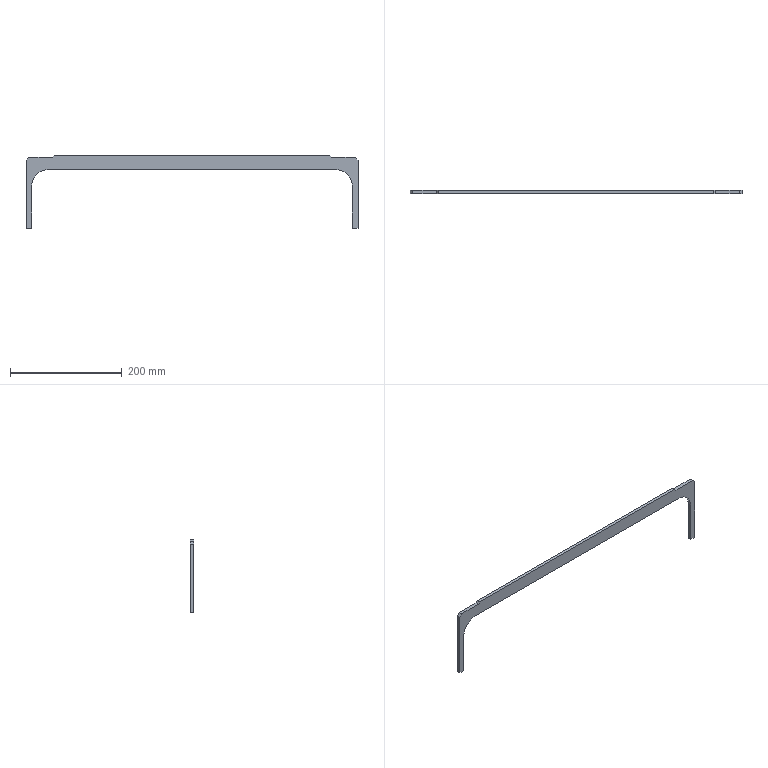Part | SolidWorks | features FlatPattern 1, SMBaseFlange 1, SheetMetal 1 | 1 solid | 18 faces | box 593.5 x 6 x 130 mm | volume 101926 mm3 | plane 16 | cylinder 2 | commonest cylinder face diameters 60 x2
STEP:
#1=CARTESIAN_POINT('',(0.,0.,0.));
#2=VERTEX_POINT('',#1);
#3=CARTESIAN_POINT('',(0.,0.,121.8));
#4=VERTEX_POINT('',#3);
#5=CARTESIAN_POINT('',(0.,0.,0.));
#6=DIRECTION('',(0.,0.,1.));
#7=VECTOR('',#6,1000.);
#8=LINE('',#5,#7);
#9=EDGE_CURVE('',#2,#4,#8,.T.);
#10=ORIENTED_EDGE('',*,*,#9,.F.);
#11=CARTESIAN_POINT('',(0.,-6.,0.));
#12=VERTEX_POINT('',#11);
#13=CARTESIAN_POINT('',(0.,-6.,0.));
#14=DIRECTION('',(0.,1.,0.));
#15=VECTOR('',#14,1000.);
#16=LINE('',#13,#15);
#17=EDGE_CURVE('',#12,#2,#16,.T.);
#18=ORIENTED_EDGE('',*,*,#17,.F.);
#19=CARTESIAN_POINT('',(0.,-6.,121.8));
#20=VERTEX_POINT('',#19);
#21=CARTESIAN_POINT('',(0.,-6.,0.));
#22=DIRECTION('',(0.,0.,1.));
#23=VECTOR('',#22,1000.);
#24=LINE('',#21,#23);
#25=EDGE_CURVE('',#12,#20,#24,.T.);
#26=ORIENTED_EDGE('',*,*,#25,.T.);
#27=CARTESIAN_POINT('',(0.,-6.,121.8));
#28=DIRECTION('',(0.,1.,0.));
#29=VECTOR('',#28,1000.);
#30=LINE('',#27,#29);
#31=EDGE_CURVE('',#20,#4,#30,.T.);
#32=ORIENTED_EDGE('',*,*,#31,.T.);
#33=EDGE_LOOP('',(#10,#18,#26,#32));
#34=FACE_OUTER_BOUND('',#33,.T.);
#35=CARTESIAN_POINT('',(0.,-6.,0.));
#36=DIRECTION('',(-1.,0.,0.));
#37=DIRECTION('',(0.,0.,1.));
#38=AXIS2_PLACEMENT_3D('',#35,#36,#37);
#39=PLANE('',#38);
#40=ADVANCED_FACE('',(#34),#39,.T.);
#41=CARTESIAN_POINT('',(10.,0.,0.));
#42=VERTEX_POINT('',#41);
#43=CARTESIAN_POINT('',(0.,0.,0.));
#44=DIRECTION('',(-1.,0.,0.));
#45=VECTOR('',#44,1000.);
#46=LINE('',#43,#45);
#47=EDGE_CURVE('',#42,#2,#46,.T.);
#48=ORIENTED_EDGE('',*,*,#47,.F.);
#49=CARTESIAN_POINT('',(10.,-6.,0.));
#50=VERTEX_POINT('',#49);
#51=CARTESIAN_POINT('',(10.,-6.,0.));
#52=DIRECTION('',(0.,1.,0.));
#53=VECTOR('',#52,1000.);
#54=LINE('',#51,#53);
#55=EDGE_CURVE('',#50,#42,#54,.T.);
#56=ORIENTED_EDGE('',*,*,#55,.F.);
#57=CARTESIAN_POINT('',(0.,-6.,0.));
#58=DIRECTION('',(-1.,0.,0.));
#59=VECTOR('',#58,1000.);
#60=LINE('',#57,#59);
#61=EDGE_CURVE('',#50,#12,#60,.T.);
#62=ORIENTED_EDGE('',*,*,#61,.T.);
#63=ORIENTED_EDGE('',*,*,#17,.T.);
#64=EDGE_LOOP('',(#48,#56,#62,#63));
#65=FACE_OUTER_BOUND('',#64,.T.);
#66=CARTESIAN_POINT('',(0.,-6.,0.));
#67=DIRECTION('',(0.,0.,-1.));
#68=DIRECTION('',(-1.,0.,0.));
#69=AXIS2_PLACEMENT_3D('',#66,#67,#68);
#70=PLANE('',#69);
#71=ADVANCED_FACE('',(#65),#70,.T.);
#72=CARTESIAN_POINT('',(10.,0.,75.));
#73=VERTEX_POINT('',#72);
#74=CARTESIAN_POINT('',(10.,0.,0.));
#75=DIRECTION('',(0.,0.,-1.));
#76=VECTOR('',#75,1000.);
#77=LINE('',#74,#76);
#78=EDGE_CURVE('',#73,#42,#77,.T.);
#79=ORIENTED_EDGE('',*,*,#78,.F.);
#80=CARTESIAN_POINT('',(10.,-6.,75.));
#81=VERTEX_POINT('',#80);
#82=CARTESIAN_POINT('',(10.,-6.,75.));
#83=DIRECTION('',(0.,1.,0.));
#84=VECTOR('',#83,1000.);
#85=LINE('',#82,#84);
#86=EDGE_CURVE('',#81,#73,#85,.T.);
#87=ORIENTED_EDGE('',*,*,#86,.F.);
#88=CARTESIAN_POINT('',(10.,-6.,0.));
#89=DIRECTION('',(0.,0.,-1.));
#90=VECTOR('',#89,1000.);
#91=LINE('',#88,#90);
#92=EDGE_CURVE('',#81,#50,#91,.T.);
#93=ORIENTED_EDGE('',*,*,#92,.T.);
#94=ORIENTED_EDGE('',*,*,#55,.T.);
#95=EDGE_LOOP('',(#79,#87,#93,#94));
#96=FACE_OUTER_BOUND('',#95,.T.);
#97=CARTESIAN_POINT('',(10.,-6.,0.));
#98=DIRECTION('',(1.,0.,0.));
#99=DIRECTION('',(0.,0.,-1.));
#100=AXIS2_PLACEMENT_3D('',#97,#98,#99);
#101=PLANE('',#100);
#102=ADVANCED_FACE('',(#96),#101,.T.);
#103=CARTESIAN_POINT('',(40.,0.,105.));
#104=VERTEX_POINT('',#103);
#105=CARTESIAN_POINT('',(40.,0.,75.));
#106=DIRECTION('',(0.,-1.,0.));
#107=DIRECTION('',(0.,0.,1.));
#108=AXIS2_PLACEMENT_3D('',#105,#106,#107);
#109=CIRCLE('',#108,30.);
#110=EDGE_CURVE('',#104,#73,#109,.T.);
#111=ORIENTED_EDGE('',*,*,#110,.F.);
#112=CARTESIAN_POINT('',(40.,-6.,105.));
#113=VERTEX_POINT('',#112);
#114=CARTESIAN_POINT('',(40.,-6.,105.));
#115=DIRECTION('',(0.,1.,0.));
#116=VECTOR('',#115,1000.);
#117=LINE('',#114,#116);
#118=EDGE_CURVE('',#113,#104,#117,.T.);
#119=ORIENTED_EDGE('',*,*,#118,.F.);
#120=CARTESIAN_POINT('',(40.,-6.,75.));
#121=DIRECTION('',(0.,-1.,0.));
#122=DIRECTION('',(0.,0.,1.));
#123=AXIS2_PLACEMENT_3D('',#120,#121,#122);
#124=CIRCLE('',#123,30.);
#125=EDGE_CURVE('',#113,#81,#124,.T.);
#126=ORIENTED_EDGE('',*,*,#125,.T.);
#127=ORIENTED_EDGE('',*,*,#86,.T.);
#128=EDGE_LOOP('',(#111,#119,#126,#127));
#129=FACE_OUTER_BOUND('',#128,.T.);
#130=CARTESIAN_POINT('',(40.,-6.,75.));
#131=DIRECTION('',(0.,1.,0.));
#132=DIRECTION('',(0.,0.,1.));
#133=AXIS2_PLACEMENT_3D('',#130,#131,#132);
#134=CYLINDRICAL_SURFACE('',#133,30.);
#135=ADVANCED_FACE('',(#129),#134,.F.);
#136=CARTESIAN_POINT('',(553.5,0.,105.));
#137=VERTEX_POINT('',#136);
#138=CARTESIAN_POINT('',(40.,0.,105.));
#139=DIRECTION('',(-1.,0.,0.));
#140=VECTOR('',#139,1000.);
#141=LINE('',#138,#140);
#142=EDGE_CURVE('',#137,#104,#141,.T.);
#143=ORIENTED_EDGE('',*,*,#142,.F.);
#144=CARTESIAN_POINT('',(553.5,-6.,105.));
#145=VERTEX_POINT('',#144);
#146=CARTESIAN_POINT('',(553.5,-6.,105.));
#147=DIRECTION('',(0.,1.,0.));
#148=VECTOR('',#147,1000.);
#149=LINE('',#146,#148);
#150=EDGE_CURVE('',#145,#137,#149,.T.);
#151=ORIENTED_EDGE('',*,*,#150,.F.);
#152=CARTESIAN_POINT('',(40.,-6.,105.));
#153=DIRECTION('',(-1.,0.,0.));
#154=VECTOR('',#153,1000.);
#155=LINE('',#152,#154);
#156=EDGE_CURVE('',#145,#113,#155,.T.);
#157=ORIENTED_EDGE('',*,*,#156,.T.);
#158=ORIENTED_EDGE('',*,*,#118,.T.);
#159=EDGE_LOOP('',(#143,#151,#157,#158));
#160=FACE_OUTER_BOUND('',#159,.T.);
#161=CARTESIAN_POINT('',(40.,-6.,105.));
#162=DIRECTION('',(0.,0.,-1.));
#163=DIRECTION('',(-1.,0.,0.));
#164=AXIS2_PLACEMENT_3D('',#161,#162,#163);
#165=PLANE('',#164);
#166=ADVANCED_FACE('',(#160),#165,.T.);
#167=CARTESIAN_POINT('',(583.5,0.,75.));
#168=VERTEX_POINT('',#167);
#169=CARTESIAN_POINT('',(553.5,0.,75.));
#170=DIRECTION('',(0.,-1.,0.));
#171=DIRECTION('',(0.,0.,1.));
#172=AXIS2_PLACEMENT_3D('',#169,#170,#171);
#173=CIRCLE('',#172,30.);
#174=EDGE_CURVE('',#168,#137,#173,.T.);
#175=ORIENTED_EDGE('',*,*,#174,.F.);
#176=CARTESIAN_POINT('',(583.5,-6.,75.));
#177=VERTEX_POINT('',#176);
#178=CARTESIAN_POINT('',(583.5,-6.,75.));
#179=DIRECTION('',(0.,1.,0.));
#180=VECTOR('',#179,1000.);
#181=LINE('',#178,#180);
#182=EDGE_CURVE('',#177,#168,#181,.T.);
#183=ORIENTED_EDGE('',*,*,#182,.F.);
#184=CARTESIAN_POINT('',(553.5,-6.,75.));
#185=DIRECTION('',(0.,-1.,0.));
#186=DIRECTION('',(0.,0.,1.));
#187=AXIS2_PLACEMENT_3D('',#184,#185,#186);
#188=CIRCLE('',#187,30.);
#189=EDGE_CURVE('',#177,#145,#188,.T.);
#190=ORIENTED_EDGE('',*,*,#189,.T.);
#191=ORIENTED_EDGE('',*,*,#150,.T.);
#192=EDGE_LOOP('',(#175,#183,#190,#191));
#193=FACE_OUTER_BOUND('',#192,.T.);
#194=CARTESIAN_POINT('',(553.5,-6.,75.));
#195=DIRECTION('',(0.,1.,0.));
#196=DIRECTION('',(0.,0.,1.));
#197=AXIS2_PLACEMENT_3D('',#194,#195,#196);
#198=CYLINDRICAL_SURFACE('',#197,30.);
#199=ADVANCED_FACE('',(#193),#198,.F.);
#200=CARTESIAN_POINT('',(583.5,0.,0.));
#201=VERTEX_POINT('',#200);
#202=CARTESIAN_POINT('',(583.5,0.,75.));
#203=DIRECTION('',(0.,0.,1.));
#204=VECTOR('',#203,1000.);
#205=LINE('',#202,#204);
#206=EDGE_CURVE('',#201,#168,#205,.T.);
#207=ORIENTED_EDGE('',*,*,#206,.F.);
#208=CARTESIAN_POINT('',(583.5,-6.,0.));
#209=VERTEX_POINT('',#208);
#210=CARTESIAN_POINT('',(583.5,-6.,0.));
#211=DIRECTION('',(0.,1.,0.));
#212=VECTOR('',#211,1000.);
#213=LINE('',#210,#212);
#214=EDGE_CURVE('',#209,#201,#213,.T.);
#215=ORIENTED_EDGE('',*,*,#214,.F.);
#216=CARTESIAN_POINT('',(583.5,-6.,75.));
#217=DIRECTION('',(0.,0.,1.));
#218=VECTOR('',#217,1000.);
#219=LINE('',#216,#218);
#220=EDGE_CURVE('',#209,#177,#219,.T.);
#221=ORIENTED_EDGE('',*,*,#220,.T.);
#222=ORIENTED_EDGE('',*,*,#182,.T.);
#223=EDGE_LOOP('',(#207,#215,#221,#222));
#224=FACE_OUTER_BOUND('',#223,.T.);
#225=CARTESIAN_POINT('',(583.5,-6.,75.));
#226=DIRECTION('',(-1.,0.,0.));
#227=DIRECTION('',(0.,0.,1.));
#228=AXIS2_PLACEMENT_3D('',#225,#226,#227);
#229=PLANE('',#228);
#230=ADVANCED_FACE('',(#224),#229,.T.);
#231=CARTESIAN_POINT('',(593.5,0.,0.));
#232=VERTEX_POINT('',#231);
#233=CARTESIAN_POINT('',(583.5,0.,0.));
#234=DIRECTION('',(-1.,0.,0.));
#235=VECTOR('',#234,1000.);
#236=LINE('',#233,#235);
#237=EDGE_CURVE('',#232,#201,#236,.T.);
#238=ORIENTED_EDGE('',*,*,#237,.F.);
#239=CARTESIAN_POINT('',(593.5,-6.,0.));
#240=VERTEX_POINT('',#239);
#241=CARTESIAN_POINT('',(593.5,-6.,0.));
#242=DIRECTION('',(0.,1.,0.));
#243=VECTOR('',#242,1000.);
#244=LINE('',#241,#243);
#245=EDGE_CURVE('',#240,#232,#244,.T.);
#246=ORIENTED_EDGE('',*,*,#245,.F.);
#247=CARTESIAN_POINT('',(583.5,-6.,0.));
#248=DIRECTION('',(-1.,0.,0.));
#249=VECTOR('',#248,1000.);
#250=LINE('',#247,#249);
#251=EDGE_CURVE('',#240,#209,#250,.T.);
#252=ORIENTED_EDGE('',*,*,#251,.T.);
#253=ORIENTED_EDGE('',*,*,#214,.T.);
#254=EDGE_LOOP('',(#238,#246,#252,#253));
#255=FACE_OUTER_BOUND('',#254,.T.);
#256=CARTESIAN_POINT('',(583.5,-6.,0.));
#257=DIRECTION('',(0.,0.,-1.));
#258=DIRECTION('',(-1.,0.,0.));
#259=AXIS2_PLACEMENT_3D('',#256,#257,#258);
#260=PLANE('',#259);
#261=ADVANCED_FACE('',(#255),#260,.T.);
#262=CARTESIAN_POINT('',(593.5,0.,121.8));
#263=VERTEX_POINT('',#262);
#264=CARTESIAN_POINT('',(593.5,0.,0.));
#265=DIRECTION('',(0.,0.,-1.));
#266=VECTOR('',#265,1000.);
#267=LINE('',#264,#266);
#268=EDGE_CURVE('',#263,#232,#267,.T.);
#269=ORIENTED_EDGE('',*,*,#268,.F.);
#270=CARTESIAN_POINT('',(593.5,-6.,121.8));
#271=VERTEX_POINT('',#270);
#272=CARTESIAN_POINT('',(593.5,-6.,121.8));
#273=DIRECTION('',(0.,1.,0.));
#274=VECTOR('',#273,1000.);
#275=LINE('',#272,#274);
#276=EDGE_CURVE('',#271,#263,#275,.T.);
#277=ORIENTED_EDGE('',*,*,#276,.F.);
#278=CARTESIAN_POINT('',(593.5,-6.,0.));
#279=DIRECTION('',(0.,0.,-1.));
#280=VECTOR('',#279,1000.);
#281=LINE('',#278,#280);
#282=EDGE_CURVE('',#271,#240,#281,.T.);
#283=ORIENTED_EDGE('',*,*,#282,.T.);
#284=ORIENTED_EDGE('',*,*,#245,.T.);
#285=EDGE_LOOP('',(#269,#277,#283,#284));
#286=FACE_OUTER_BOUND('',#285,.T.);
#287=CARTESIAN_POINT('',(593.5,-6.,0.));
#288=DIRECTION('',(1.,0.,0.));
#289=DIRECTION('',(0.,0.,-1.));
#290=AXIS2_PLACEMENT_3D('',#287,#288,#289);
#291=PLANE('',#290);
#292=ADVANCED_FACE('',(#286),#291,.T.);
#293=CARTESIAN_POINT('',(588.5,0.,126.8));
#294=VERTEX_POINT('',#293);
#295=CARTESIAN_POINT('',(593.5,0.,121.8));
#296=DIRECTION('',(0.7071,0.,-0.7071));
#297=VECTOR('',#296,1000.);
#298=LINE('',#295,#297);
#299=EDGE_CURVE('',#294,#263,#298,.T.);
#300=ORIENTED_EDGE('',*,*,#299,.F.);
#301=CARTESIAN_POINT('',(588.5,-6.,126.8));
#302=VERTEX_POINT('',#301);
#303=CARTESIAN_POINT('',(588.5,-6.,126.8));
#304=DIRECTION('',(0.,1.,0.));
#305=VECTOR('',#304,1000.);
#306=LINE('',#303,#305);
#307=EDGE_CURVE('',#302,#294,#306,.T.);
#308=ORIENTED_EDGE('',*,*,#307,.F.);
#309=CARTESIAN_POINT('',(593.5,-6.,121.8));
#310=DIRECTION('',(0.7071,0.,-0.7071));
#311=VECTOR('',#310,1000.);
#312=LINE('',#309,#311);
#313=EDGE_CURVE('',#302,#271,#312,.T.);
#314=ORIENTED_EDGE('',*,*,#313,.T.);
#315=ORIENTED_EDGE('',*,*,#276,.T.);
#316=EDGE_LOOP('',(#300,#308,#314,#315));
#317=FACE_OUTER_BOUND('',#316,.T.);
#318=CARTESIAN_POINT('',(593.5,-6.,121.8));
#319=DIRECTION('',(0.7071,0.,0.7071));
#320=DIRECTION('',(0.7071,0.,-0.7071));
#321=AXIS2_PLACEMENT_3D('',#318,#319,#320);
#322=PLANE('',#321);
#323=ADVANCED_FACE('',(#317),#322,.T.);
#324=CARTESIAN_POINT('',(546.5,0.,126.8));
#325=VERTEX_POINT('',#324);
#326=CARTESIAN_POINT('',(588.5,0.,126.8));
#327=DIRECTION('',(1.,0.,0.));
#328=VECTOR('',#327,1000.);
#329=LINE('',#326,#328);
#330=EDGE_CURVE('',#325,#294,#329,.T.);
#331=ORIENTED_EDGE('',*,*,#330,.F.);
#332=CARTESIAN_POINT('',(546.5,-6.,126.8));
#333=VERTEX_POINT('',#332);
#334=CARTESIAN_POINT('',(546.5,-6.,126.8));
#335=DIRECTION('',(0.,1.,0.));
#336=VECTOR('',#335,1000.);
#337=LINE('',#334,#336);
#338=EDGE_CURVE('',#333,#325,#337,.T.);
#339=ORIENTED_EDGE('',*,*,#338,.F.);
#340=CARTESIAN_POINT('',(588.5,-6.,126.8));
#341=DIRECTION('',(1.,0.,0.));
#342=VECTOR('',#341,1000.);
#343=LINE('',#340,#342);
#344=EDGE_CURVE('',#333,#302,#343,.T.);
#345=ORIENTED_EDGE('',*,*,#344,.T.);
#346=ORIENTED_EDGE('',*,*,#307,.T.);
#347=EDGE_LOOP('',(#331,#339,#345,#346));
#348=FACE_OUTER_BOUND('',#347,.T.);
#349=CARTESIAN_POINT('',(588.5,-6.,126.8));
#350=DIRECTION('',(0.,0.,1.));
#351=DIRECTION('',(1.,0.,0.));
#352=AXIS2_PLACEMENT_3D('',#349,#350,#351);
#353=PLANE('',#352);
#354=ADVANCED_FACE('',(#348),#353,.T.);
#355=CARTESIAN_POINT('',(543.3,0.,130.));
#356=VERTEX_POINT('',#355);
#357=CARTESIAN_POINT('',(546.5,0.,126.8));
#358=DIRECTION('',(0.7071,0.,-0.7071));
#359=VECTOR('',#358,1000.);
#360=LINE('',#357,#359);
#361=EDGE_CURVE('',#356,#325,#360,.T.);
#362=ORIENTED_EDGE('',*,*,#361,.F.);
#363=CARTESIAN_POINT('',(543.3,-6.,130.));
#364=VERTEX_POINT('',#363);
#365=CARTESIAN_POINT('',(543.3,-6.,130.));
#366=DIRECTION('',(0.,1.,0.));
#367=VECTOR('',#366,1000.);
#368=LINE('',#365,#367);
#369=EDGE_CURVE('',#364,#356,#368,.T.);
#370=ORIENTED_EDGE('',*,*,#369,.F.);
#371=CARTESIAN_POINT('',(546.5,-6.,126.8));
#372=DIRECTION('',(0.7071,0.,-0.7071));
#373=VECTOR('',#372,1000.);
#374=LINE('',#371,#373);
#375=EDGE_CURVE('',#364,#333,#374,.T.);
#376=ORIENTED_EDGE('',*,*,#375,.T.);
#377=ORIENTED_EDGE('',*,*,#338,.T.);
#378=EDGE_LOOP('',(#362,#370,#376,#377));
#379=FACE_OUTER_BOUND('',#378,.T.);
#380=CARTESIAN_POINT('',(546.5,-6.,126.8));
#381=DIRECTION('',(0.7071,0.,0.7071));
#382=DIRECTION('',(0.7071,0.,-0.7071));
#383=AXIS2_PLACEMENT_3D('',#380,#381,#382);
#384=PLANE('',#383);
#385=ADVANCED_FACE('',(#379),#384,.T.);
#386=CARTESIAN_POINT('',(50.2,0.,130.));
#387=VERTEX_POINT('',#386);
#388=CARTESIAN_POINT('',(50.2,0.,130.));
#389=DIRECTION('',(1.,0.,0.));
#390=VECTOR('',#389,1000.);
#391=LINE('',#388,#390);
#392=EDGE_CURVE('',#387,#356,#391,.T.);
#393=ORIENTED_EDGE('',*,*,#392,.F.);
#394=CARTESIAN_POINT('',(50.2,-6.,130.));
#395=VERTEX_POINT('',#394);
#396=CARTESIAN_POINT('',(50.2,-6.,130.));
#397=DIRECTION('',(0.,1.,0.));
#398=VECTOR('',#397,1000.);
#399=LINE('',#396,#398);
#400=EDGE_CURVE('',#395,#387,#399,.T.);
#401=ORIENTED_EDGE('',*,*,#400,.F.);
#402=CARTESIAN_POINT('',(50.2,-6.,130.));
#403=DIRECTION('',(1.,0.,0.));
#404=VECTOR('',#403,1000.);
#405=LINE('',#402,#404);
#406=EDGE_CURVE('',#395,#364,#405,.T.);
#407=ORIENTED_EDGE('',*,*,#406,.T.);
#408=ORIENTED_EDGE('',*,*,#369,.T.);
#409=EDGE_LOOP('',(#393,#401,#407,#408));
#410=FACE_OUTER_BOUND('',#409,.T.);
#411=CARTESIAN_POINT('',(50.2,-6.,130.));
#412=DIRECTION('',(0.,0.,1.));
#413=DIRECTION('',(1.,0.,0.));
#414=AXIS2_PLACEMENT_3D('',#411,#412,#413);
#415=PLANE('',#414);
#416=ADVANCED_FACE('',(#410),#415,.T.);
#417=CARTESIAN_POINT('',(47.,0.,126.8));
#418=VERTEX_POINT('',#417);
#419=CARTESIAN_POINT('',(47.,0.,126.8));
#420=DIRECTION('',(0.7071,0.,0.7071));
#421=VECTOR('',#420,1000.);
#422=LINE('',#419,#421);
#423=EDGE_CURVE('',#418,#387,#422,.T.);
#424=ORIENTED_EDGE('',*,*,#423,.F.);
#425=CARTESIAN_POINT('',(47.,-6.,126.8));
#426=VERTEX_POINT('',#425);
#427=CARTESIAN_POINT('',(47.,-6.,126.8));
#428=DIRECTION('',(0.,1.,0.));
#429=VECTOR('',#428,1000.);
#430=LINE('',#427,#429);
#431=EDGE_CURVE('',#426,#418,#430,.T.);
#432=ORIENTED_EDGE('',*,*,#431,.F.);
#433=CARTESIAN_POINT('',(47.,-6.,126.8));
#434=DIRECTION('',(0.7071,0.,0.7071));
#435=VECTOR('',#434,1000.);
#436=LINE('',#433,#435);
#437=EDGE_CURVE('',#426,#395,#436,.T.);
#438=ORIENTED_EDGE('',*,*,#437,.T.);
#439=ORIENTED_EDGE('',*,*,#400,.T.);
#440=EDGE_LOOP('',(#424,#432,#438,#439));
#441=FACE_OUTER_BOUND('',#440,.T.);
#442=CARTESIAN_POINT('',(47.,-6.,126.8));
#443=DIRECTION('',(-0.7071,0.,0.7071));
#444=DIRECTION('',(0.7071,0.,0.7071));
#445=AXIS2_PLACEMENT_3D('',#442,#443,#444);
#446=PLANE('',#445);
#447=ADVANCED_FACE('',(#441),#446,.T.);
#448=CARTESIAN_POINT('',(5.,0.,126.8));
#449=VERTEX_POINT('',#448);
#450=CARTESIAN_POINT('',(5.,0.,126.8));
#451=DIRECTION('',(1.,0.,0.));
#452=VECTOR('',#451,1000.);
#453=LINE('',#450,#452);
#454=EDGE_CURVE('',#449,#418,#453,.T.);
#455=ORIENTED_EDGE('',*,*,#454,.F.);
#456=CARTESIAN_POINT('',(5.,-6.,126.8));
#457=VERTEX_POINT('',#456);
#458=CARTESIAN_POINT('',(5.,-6.,126.8));
#459=DIRECTION('',(0.,1.,0.));
#460=VECTOR('',#459,1000.);
#461=LINE('',#458,#460);
#462=EDGE_CURVE('',#457,#449,#461,.T.);
#463=ORIENTED_EDGE('',*,*,#462,.F.);
#464=CARTESIAN_POINT('',(5.,-6.,126.8));
#465=DIRECTION('',(1.,0.,0.));
#466=VECTOR('',#465,1000.);
#467=LINE('',#464,#466);
#468=EDGE_CURVE('',#457,#426,#467,.T.);
#469=ORIENTED_EDGE('',*,*,#468,.T.);
#470=ORIENTED_EDGE('',*,*,#431,.T.);
#471=EDGE_LOOP('',(#455,#463,#469,#470));
#472=FACE_OUTER_BOUND('',#471,.T.);
#473=CARTESIAN_POINT('',(5.,-6.,126.8));
#474=DIRECTION('',(0.,0.,1.));
#475=DIRECTION('',(1.,0.,0.));
#476=AXIS2_PLACEMENT_3D('',#473,#474,#475);
#477=PLANE('',#476);
#478=ADVANCED_FACE('',(#472),#477,.T.);
#479=CARTESIAN_POINT('',(0.,0.,121.8));
#480=DIRECTION('',(0.7071,0.,0.7071));
#481=VECTOR('',#480,1000.);
#482=LINE('',#479,#481);
#483=EDGE_CURVE('',#4,#449,#482,.T.);
#484=ORIENTED_EDGE('',*,*,#483,.F.);
#485=ORIENTED_EDGE('',*,*,#31,.F.);
#486=CARTESIAN_POINT('',(0.,-6.,121.8));
#487=DIRECTION('',(0.7071,0.,0.7071));
#488=VECTOR('',#487,1000.);
#489=LINE('',#486,#488);
#490=EDGE_CURVE('',#20,#457,#489,.T.);
#491=ORIENTED_EDGE('',*,*,#490,.T.);
#492=ORIENTED_EDGE('',*,*,#462,.T.);
#493=EDGE_LOOP('',(#484,#485,#491,#492));
#494=FACE_OUTER_BOUND('',#493,.T.);
#495=CARTESIAN_POINT('',(0.,-6.,121.8));
#496=DIRECTION('',(-0.7071,0.,0.7071));
#497=DIRECTION('',(0.7071,0.,0.7071));
#498=AXIS2_PLACEMENT_3D('',#495,#496,#497);
#499=PLANE('',#498);
#500=ADVANCED_FACE('',(#494),#499,.T.);
#501=ORIENTED_EDGE('',*,*,#25,.F.);
#502=ORIENTED_EDGE('',*,*,#61,.F.);
#503=ORIENTED_EDGE('',*,*,#92,.F.);
#504=ORIENTED_EDGE('',*,*,#125,.F.);
#505=ORIENTED_EDGE('',*,*,#156,.F.);
#506=ORIENTED_EDGE('',*,*,#189,.F.);
#507=ORIENTED_EDGE('',*,*,#220,.F.);
#508=ORIENTED_EDGE('',*,*,#251,.F.);
#509=ORIENTED_EDGE('',*,*,#282,.F.);
#510=ORIENTED_EDGE('',*,*,#313,.F.);
#511=ORIENTED_EDGE('',*,*,#344,.F.);
#512=ORIENTED_EDGE('',*,*,#375,.F.);
#513=ORIENTED_EDGE('',*,*,#406,.F.);
#514=ORIENTED_EDGE('',*,*,#437,.F.);
#515=ORIENTED_EDGE('',*,*,#468,.F.);
#516=ORIENTED_EDGE('',*,*,#490,.F.);
#517=EDGE_LOOP('',(#501,#502,#503,#504,#505,#506,#507,#508,#509,#510,#511,#512,#513,#514,#515,#516));
#518=FACE_OUTER_BOUND('',#517,.T.);
#519=CARTESIAN_POINT('',(553.5,-6.,75.));
#520=DIRECTION('',(0.,1.,0.));
#521=DIRECTION('',(0.,0.,1.));
#522=AXIS2_PLACEMENT_3D('',#519,#520,#521);
#523=PLANE('',#522);
#524=ADVANCED_FACE('',(#518),#523,.F.);
#525=ORIENTED_EDGE('',*,*,#9,.T.);
#526=ORIENTED_EDGE('',*,*,#483,.T.);
#527=ORIENTED_EDGE('',*,*,#454,.T.);
#528=ORIENTED_EDGE('',*,*,#423,.T.);
#529=ORIENTED_EDGE('',*,*,#392,.T.);
#530=ORIENTED_EDGE('',*,*,#361,.T.);
#531=ORIENTED_EDGE('',*,*,#330,.T.);
#532=ORIENTED_EDGE('',*,*,#299,.T.);
#533=ORIENTED_EDGE('',*,*,#268,.T.);
#534=ORIENTED_EDGE('',*,*,#237,.T.);
#535=ORIENTED_EDGE('',*,*,#206,.T.);
#536=ORIENTED_EDGE('',*,*,#174,.T.);
#537=ORIENTED_EDGE('',*,*,#142,.T.);
#538=ORIENTED_EDGE('',*,*,#110,.T.);
#539=ORIENTED_EDGE('',*,*,#78,.T.);
#540=ORIENTED_EDGE('',*,*,#47,.T.);
#541=EDGE_LOOP('',(#525,#526,#527,#528,#529,#530,#531,#532,#533,#534,#535,#536,#537,#538,#539,#540));
#542=FACE_OUTER_BOUND('',#541,.T.);
#543=CARTESIAN_POINT('',(553.5,0.,75.));
#544=DIRECTION('',(0.,1.,0.));
#545=DIRECTION('',(0.,0.,1.));
#546=AXIS2_PLACEMENT_3D('',#543,#544,#545);
#547=PLANE('',#546);
#548=ADVANCED_FACE('',(#542),#547,.T.);
#549=CLOSED_SHELL('',(#40,#71,#102,#135,#166,#199,#230,#261,#292,#323,#354,#385,#416,#447,#478,#500,#524,#548));
#550=MANIFOLD_SOLID_BREP('',#549);
#551=CARTESIAN_POINT('',(0.,0.,0.));
#552=DIRECTION('',(0.,0.,1.));
#553=DIRECTION('',(1.,0.,0.));
#554=AXIS2_PLACEMENT_3D('',#551,#552,#553);
#555=(LENGTH_UNIT()NAMED_UNIT(*)SI_UNIT(.MILLI.,.METRE.));
#556=UNCERTAINTY_MEASURE_WITH_UNIT(LENGTH_MEASURE(0.00001),#555,'','');
#557=(NAMED_UNIT(*)PLANE_ANGLE_UNIT()SI_UNIT($,.RADIAN.));
#558=(NAMED_UNIT(*)SI_UNIT($,.STERADIAN.)SOLID_ANGLE_UNIT());
#559=(GEOMETRIC_REPRESENTATION_CONTEXT(3)GLOBAL_UNCERTAINTY_ASSIGNED_CONTEXT((#556))GLOBAL_UNIT_ASSIGNED_CONTEXT((#555,#557,#558))REPRESENTATION_CONTEXT('',''));
#560=ADVANCED_BREP_SHAPE_REPRESENTATION('',(#550,#554),#559);